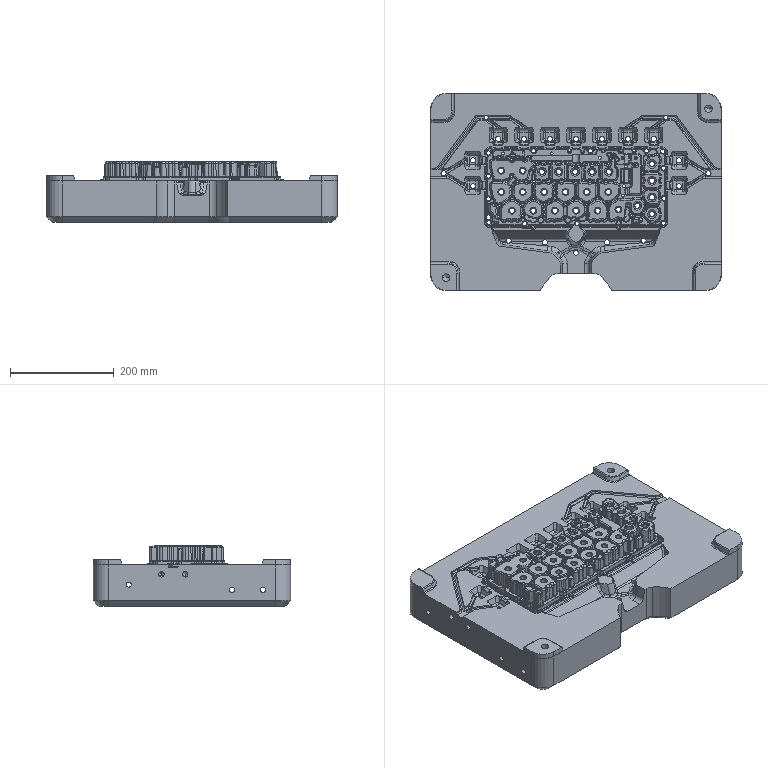Part | SolidWorks | features BaseBody 1 | 1 solid | 5417 faces | volume 16717286 mm3 | cylinder 1628 | torus 1338 | plane 871 | spline 749 | cone 718 | sphere 113 | commonest cylinder face diameters 1.005 x265 10 x207 4.022 x144 4 x133 6 x128 1.006 x127